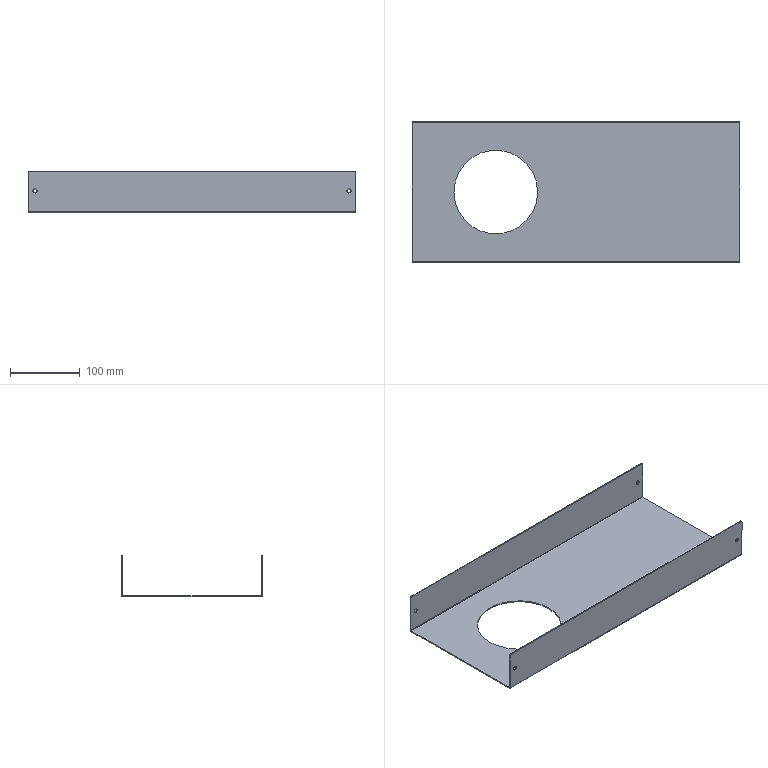Part | SolidWorks | features HoleWzd 2, Cut 1, EdgeFlange 1, Fillet 1, FlatPattern 1, SMBaseFlange 1, SheetMetal 1 | 1 solid | 36 faces | box 470 x 203 x 60 mm | volume 207704 mm3 | cylinder 18 | plane 18 | commonest cylinder face diameters 6 x8 4 x6 1 x2 120 x2
STEP:
#1=CARTESIAN_POINT('',(225.,101.5,33.));
#2=VERTEX_POINT('',#1);
#3=CARTESIAN_POINT('',(225.,101.5,27.));
#4=VERTEX_POINT('',#3);
#5=CARTESIAN_POINT('',(225.,101.5,30.));
#6=DIRECTION('',(0.,-1.,0.));
#7=DIRECTION('',(0.,0.,-1.));
#8=AXIS2_PLACEMENT_3D('',#5,#6,#7);
#9=CIRCLE('',#8,3.);
#10=EDGE_CURVE('',#2,#4,#9,.T.);
#11=ORIENTED_EDGE('',*,*,#10,.F.);
#12=CARTESIAN_POINT('',(225.,100.,33.));
#13=VERTEX_POINT('',#12);
#14=CARTESIAN_POINT('',(225.,100.,33.));
#15=DIRECTION('',(0.,-1.,0.));
#16=VECTOR('',#15,1000.);
#17=LINE('',#14,#16);
#18=EDGE_CURVE('',#2,#13,#17,.T.);
#19=ORIENTED_EDGE('',*,*,#18,.T.);
#20=CARTESIAN_POINT('',(225.,100.,27.));
#21=VERTEX_POINT('',#20);
#22=CARTESIAN_POINT('',(225.,100.,30.));
#23=DIRECTION('',(0.,-1.,0.));
#24=DIRECTION('',(0.,0.,-1.));
#25=AXIS2_PLACEMENT_3D('',#22,#23,#24);
#26=CIRCLE('',#25,3.);
#27=EDGE_CURVE('',#13,#21,#26,.T.);
#28=ORIENTED_EDGE('',*,*,#27,.T.);
#29=CARTESIAN_POINT('',(225.,100.,27.));
#30=DIRECTION('',(0.,-1.,0.));
#31=VECTOR('',#30,1000.);
#32=LINE('',#29,#31);
#33=EDGE_CURVE('',#4,#21,#32,.T.);
#34=ORIENTED_EDGE('',*,*,#33,.F.);
#35=EDGE_LOOP('',(#11,#19,#28,#34));
#36=FACE_OUTER_BOUND('',#35,.T.);
#37=CARTESIAN_POINT('',(225.,100.,30.));
#38=DIRECTION('',(0.,-1.,0.));
#39=DIRECTION('',(0.,0.,-1.));
#40=AXIS2_PLACEMENT_3D('',#37,#38,#39);
#41=CYLINDRICAL_SURFACE('',#40,3.);
#42=ADVANCED_FACE('',(#36),#41,.F.);
#43=CARTESIAN_POINT('',(-225.,101.5,33.));
#44=VERTEX_POINT('',#43);
#45=CARTESIAN_POINT('',(-225.,101.5,27.));
#46=VERTEX_POINT('',#45);
#47=CARTESIAN_POINT('',(-225.,101.5,30.));
#48=DIRECTION('',(0.,-1.,0.));
#49=DIRECTION('',(0.,0.,-1.));
#50=AXIS2_PLACEMENT_3D('',#47,#48,#49);
#51=CIRCLE('',#50,3.);
#52=EDGE_CURVE('',#44,#46,#51,.T.);
#53=ORIENTED_EDGE('',*,*,#52,.F.);
#54=CARTESIAN_POINT('',(-225.,100.,33.));
#55=VERTEX_POINT('',#54);
#56=CARTESIAN_POINT('',(-225.,100.,33.));
#57=DIRECTION('',(0.,-1.,0.));
#58=VECTOR('',#57,1000.);
#59=LINE('',#56,#58);
#60=EDGE_CURVE('',#44,#55,#59,.T.);
#61=ORIENTED_EDGE('',*,*,#60,.T.);
#62=CARTESIAN_POINT('',(-225.,100.,27.));
#63=VERTEX_POINT('',#62);
#64=CARTESIAN_POINT('',(-225.,100.,30.));
#65=DIRECTION('',(0.,-1.,0.));
#66=DIRECTION('',(0.,0.,-1.));
#67=AXIS2_PLACEMENT_3D('',#64,#65,#66);
#68=CIRCLE('',#67,3.);
#69=EDGE_CURVE('',#55,#63,#68,.T.);
#70=ORIENTED_EDGE('',*,*,#69,.T.);
#71=CARTESIAN_POINT('',(-225.,100.,27.));
#72=DIRECTION('',(0.,-1.,0.));
#73=VECTOR('',#72,1000.);
#74=LINE('',#71,#73);
#75=EDGE_CURVE('',#46,#63,#74,.T.);
#76=ORIENTED_EDGE('',*,*,#75,.F.);
#77=EDGE_LOOP('',(#53,#61,#70,#76));
#78=FACE_OUTER_BOUND('',#77,.T.);
#79=CARTESIAN_POINT('',(-225.,100.,30.));
#80=DIRECTION('',(0.,-1.,0.));
#81=DIRECTION('',(0.,0.,-1.));
#82=AXIS2_PLACEMENT_3D('',#79,#80,#81);
#83=CYLINDRICAL_SURFACE('',#82,3.);
#84=ADVANCED_FACE('',(#78),#83,.F.);
#85=CARTESIAN_POINT('',(-225.,-101.5,27.));
#86=VERTEX_POINT('',#85);
#87=CARTESIAN_POINT('',(-225.,-101.5,33.));
#88=VERTEX_POINT('',#87);
#89=CARTESIAN_POINT('',(-225.,-101.5,30.));
#90=DIRECTION('',(0.,1.,0.));
#91=DIRECTION('',(0.,0.,1.));
#92=AXIS2_PLACEMENT_3D('',#89,#90,#91);
#93=CIRCLE('',#92,3.);
#94=EDGE_CURVE('',#86,#88,#93,.T.);
#95=ORIENTED_EDGE('',*,*,#94,.F.);
#96=CARTESIAN_POINT('',(-225.,-100.,27.));
#97=VERTEX_POINT('',#96);
#98=CARTESIAN_POINT('',(-225.,-100.,27.));
#99=DIRECTION('',(0.,1.,0.));
#100=VECTOR('',#99,1000.);
#101=LINE('',#98,#100);
#102=EDGE_CURVE('',#86,#97,#101,.T.);
#103=ORIENTED_EDGE('',*,*,#102,.T.);
#104=CARTESIAN_POINT('',(-225.,-100.,33.));
#105=VERTEX_POINT('',#104);
#106=CARTESIAN_POINT('',(-225.,-100.,30.));
#107=DIRECTION('',(0.,1.,0.));
#108=DIRECTION('',(0.,0.,1.));
#109=AXIS2_PLACEMENT_3D('',#106,#107,#108);
#110=CIRCLE('',#109,3.);
#111=EDGE_CURVE('',#97,#105,#110,.T.);
#112=ORIENTED_EDGE('',*,*,#111,.T.);
#113=CARTESIAN_POINT('',(-225.,-100.,33.));
#114=DIRECTION('',(0.,1.,0.));
#115=VECTOR('',#114,1000.);
#116=LINE('',#113,#115);
#117=EDGE_CURVE('',#88,#105,#116,.T.);
#118=ORIENTED_EDGE('',*,*,#117,.F.);
#119=EDGE_LOOP('',(#95,#103,#112,#118));
#120=FACE_OUTER_BOUND('',#119,.T.);
#121=CARTESIAN_POINT('',(-225.,-100.,30.));
#122=DIRECTION('',(0.,1.,0.));
#123=DIRECTION('',(0.,0.,1.));
#124=AXIS2_PLACEMENT_3D('',#121,#122,#123);
#125=CYLINDRICAL_SURFACE('',#124,3.);
#126=ADVANCED_FACE('',(#120),#125,.F.);
#127=CARTESIAN_POINT('',(225.,-101.5,27.));
#128=VERTEX_POINT('',#127);
#129=CARTESIAN_POINT('',(225.,-101.5,33.));
#130=VERTEX_POINT('',#129);
#131=CARTESIAN_POINT('',(225.,-101.5,30.));
#132=DIRECTION('',(0.,1.,0.));
#133=DIRECTION('',(0.,0.,1.));
#134=AXIS2_PLACEMENT_3D('',#131,#132,#133);
#135=CIRCLE('',#134,3.);
#136=EDGE_CURVE('',#128,#130,#135,.T.);
#137=ORIENTED_EDGE('',*,*,#136,.F.);
#138=CARTESIAN_POINT('',(225.,-100.,27.));
#139=VERTEX_POINT('',#138);
#140=CARTESIAN_POINT('',(225.,-100.,27.));
#141=DIRECTION('',(0.,1.,0.));
#142=VECTOR('',#141,1000.);
#143=LINE('',#140,#142);
#144=EDGE_CURVE('',#128,#139,#143,.T.);
#145=ORIENTED_EDGE('',*,*,#144,.T.);
#146=CARTESIAN_POINT('',(225.,-100.,33.));
#147=VERTEX_POINT('',#146);
#148=CARTESIAN_POINT('',(225.,-100.,30.));
#149=DIRECTION('',(0.,1.,0.));
#150=DIRECTION('',(0.,0.,1.));
#151=AXIS2_PLACEMENT_3D('',#148,#149,#150);
#152=CIRCLE('',#151,3.);
#153=EDGE_CURVE('',#139,#147,#152,.T.);
#154=ORIENTED_EDGE('',*,*,#153,.T.);
#155=CARTESIAN_POINT('',(225.,-100.,33.));
#156=DIRECTION('',(0.,1.,0.));
#157=VECTOR('',#156,1000.);
#158=LINE('',#155,#157);
#159=EDGE_CURVE('',#130,#147,#158,.T.);
#160=ORIENTED_EDGE('',*,*,#159,.F.);
#161=EDGE_LOOP('',(#137,#145,#154,#160));
#162=FACE_OUTER_BOUND('',#161,.T.);
#163=CARTESIAN_POINT('',(225.,-100.,30.));
#164=DIRECTION('',(0.,1.,0.));
#165=DIRECTION('',(0.,0.,1.));
#166=AXIS2_PLACEMENT_3D('',#163,#164,#165);
#167=CYLINDRICAL_SURFACE('',#166,3.);
#168=ADVANCED_FACE('',(#162),#167,.F.);
#169=CARTESIAN_POINT('',(-175.,0.,0.));
#170=VERTEX_POINT('',#169);
#171=CARTESIAN_POINT('',(-55.,0.,0.));
#172=VERTEX_POINT('',#171);
#173=CARTESIAN_POINT('',(-115.,0.,0.));
#174=DIRECTION('',(0.,0.,1.));
#175=DIRECTION('',(1.,0.,0.));
#176=AXIS2_PLACEMENT_3D('',#173,#174,#175);
#177=CIRCLE('',#176,60.);
#178=EDGE_CURVE('',#170,#172,#177,.T.);
#179=ORIENTED_EDGE('',*,*,#178,.T.);
#180=CARTESIAN_POINT('',(-55.,0.,-1.5));
#181=VERTEX_POINT('',#180);
#182=CARTESIAN_POINT('',(-55.,0.,8.5));
#183=DIRECTION('',(0.,0.,-1.));
#184=VECTOR('',#183,1000.);
#185=LINE('',#182,#184);
#186=EDGE_CURVE('',#172,#181,#185,.T.);
#187=ORIENTED_EDGE('',*,*,#186,.T.);
#188=CARTESIAN_POINT('',(-175.,0.,-1.5));
#189=VERTEX_POINT('',#188);
#190=CARTESIAN_POINT('',(-115.,0.,-1.5));
#191=DIRECTION('',(0.,0.,-1.));
#192=DIRECTION('',(-1.,0.,0.));
#193=AXIS2_PLACEMENT_3D('',#190,#191,#192);
#194=CIRCLE('',#193,60.);
#195=EDGE_CURVE('',#181,#189,#194,.T.);
#196=ORIENTED_EDGE('',*,*,#195,.T.);
#197=CARTESIAN_POINT('',(-175.,0.,8.5));
#198=DIRECTION('',(0.,0.,-1.));
#199=VECTOR('',#198,1000.);
#200=LINE('',#197,#199);
#201=EDGE_CURVE('',#170,#189,#200,.T.);
#202=ORIENTED_EDGE('',*,*,#201,.F.);
#203=EDGE_LOOP('',(#179,#187,#196,#202));
#204=FACE_OUTER_BOUND('',#203,.T.);
#205=CARTESIAN_POINT('',(-115.,0.,8.5));
#206=DIRECTION('',(0.,0.,-1.));
#207=DIRECTION('',(-1.,0.,0.));
#208=AXIS2_PLACEMENT_3D('',#205,#206,#207);
#209=CYLINDRICAL_SURFACE('',#208,60.);
#210=ADVANCED_FACE('',(#204),#209,.F.);
#211=CARTESIAN_POINT('',(-115.,0.,-1.5));
#212=DIRECTION('',(0.,0.,-1.));
#213=DIRECTION('',(-1.,0.,0.));
#214=AXIS2_PLACEMENT_3D('',#211,#212,#213);
#215=CIRCLE('',#214,60.);
#216=EDGE_CURVE('',#189,#181,#215,.T.);
#217=ORIENTED_EDGE('',*,*,#216,.F.);
#218=ORIENTED_EDGE('',*,*,#195,.F.);
#219=EDGE_LOOP('',(#217,#218));
#220=FACE_BOUND('',#219,.T.);
#221=CARTESIAN_POINT('',(235.,-99.5,-1.5));
#222=VERTEX_POINT('',#221);
#223=CARTESIAN_POINT('',(-235.,-99.5,-1.5));
#224=VERTEX_POINT('',#223);
#225=CARTESIAN_POINT('',(235.,-99.5,-1.5));
#226=DIRECTION('',(-1.,0.,0.));
#227=VECTOR('',#226,1000.);
#228=LINE('',#225,#227);
#229=EDGE_CURVE('',#222,#224,#228,.T.);
#230=ORIENTED_EDGE('',*,*,#229,.T.);
#231=CARTESIAN_POINT('',(-235.,99.5,-1.5));
#232=VERTEX_POINT('',#231);
#233=CARTESIAN_POINT('',(-235.,100.,-1.5));
#234=DIRECTION('',(0.,-1.,0.));
#235=VECTOR('',#234,1000.);
#236=LINE('',#233,#235);
#237=EDGE_CURVE('',#232,#224,#236,.T.);
#238=ORIENTED_EDGE('',*,*,#237,.F.);
#239=CARTESIAN_POINT('',(235.,99.5,-1.5));
#240=VERTEX_POINT('',#239);
#241=CARTESIAN_POINT('',(-235.,99.5,-1.5));
#242=DIRECTION('',(1.,0.,0.));
#243=VECTOR('',#242,1000.);
#244=LINE('',#241,#243);
#245=EDGE_CURVE('',#232,#240,#244,.T.);
#246=ORIENTED_EDGE('',*,*,#245,.T.);
#247=CARTESIAN_POINT('',(235.,100.,-1.5));
#248=DIRECTION('',(0.,1.,0.));
#249=VECTOR('',#248,1000.);
#250=LINE('',#247,#249);
#251=EDGE_CURVE('',#222,#240,#250,.T.);
#252=ORIENTED_EDGE('',*,*,#251,.F.);
#253=EDGE_LOOP('',(#230,#238,#246,#252));
#254=FACE_OUTER_BOUND('',#253,.T.);
#255=CARTESIAN_POINT('',(0.,0.,-1.5));
#256=DIRECTION('',(0.,0.,1.));
#257=DIRECTION('',(1.,0.,0.));
#258=AXIS2_PLACEMENT_3D('',#255,#256,#257);
#259=PLANE('',#258);
#260=ADVANCED_FACE('',(#220,#254),#259,.F.);
#261=ORIENTED_EDGE('',*,*,#178,.F.);
#262=CARTESIAN_POINT('',(-115.,0.,0.));
#263=DIRECTION('',(0.,0.,1.));
#264=DIRECTION('',(1.,0.,0.));
#265=AXIS2_PLACEMENT_3D('',#262,#263,#264);
#266=CIRCLE('',#265,60.);
#267=EDGE_CURVE('',#172,#170,#266,.T.);
#268=ORIENTED_EDGE('',*,*,#267,.F.);
#269=EDGE_LOOP('',(#261,#268));
#270=FACE_BOUND('',#269,.T.);
#271=CARTESIAN_POINT('',(-235.,99.5,0.));
#272=VERTEX_POINT('',#271);
#273=CARTESIAN_POINT('',(-235.,-99.5,0.));
#274=VERTEX_POINT('',#273);
#275=CARTESIAN_POINT('',(-235.,100.,0.));
#276=DIRECTION('',(0.,-1.,0.));
#277=VECTOR('',#276,1000.);
#278=LINE('',#275,#277);
#279=EDGE_CURVE('',#272,#274,#278,.T.);
#280=ORIENTED_EDGE('',*,*,#279,.T.);
#281=CARTESIAN_POINT('',(235.,-99.5,0.));
#282=VERTEX_POINT('',#281);
#283=CARTESIAN_POINT('',(235.,-99.5,0.));
#284=DIRECTION('',(-1.,0.,0.));
#285=VECTOR('',#284,1000.);
#286=LINE('',#283,#285);
#287=EDGE_CURVE('',#282,#274,#286,.T.);
#288=ORIENTED_EDGE('',*,*,#287,.F.);
#289=CARTESIAN_POINT('',(235.,99.5,0.));
#290=VERTEX_POINT('',#289);
#291=CARTESIAN_POINT('',(235.,100.,0.));
#292=DIRECTION('',(0.,1.,0.));
#293=VECTOR('',#292,1000.);
#294=LINE('',#291,#293);
#295=EDGE_CURVE('',#282,#290,#294,.T.);
#296=ORIENTED_EDGE('',*,*,#295,.T.);
#297=CARTESIAN_POINT('',(-235.,99.5,0.));
#298=DIRECTION('',(1.,0.,0.));
#299=VECTOR('',#298,1000.);
#300=LINE('',#297,#299);
#301=EDGE_CURVE('',#272,#290,#300,.T.);
#302=ORIENTED_EDGE('',*,*,#301,.F.);
#303=EDGE_LOOP('',(#280,#288,#296,#302));
#304=FACE_OUTER_BOUND('',#303,.T.);
#305=CARTESIAN_POINT('',(0.,0.,0.));
#306=DIRECTION('',(0.,0.,1.));
#307=DIRECTION('',(1.,0.,0.));
#308=AXIS2_PLACEMENT_3D('',#305,#306,#307);
#309=PLANE('',#308);
#310=ADVANCED_FACE('',(#270,#304),#309,.T.);
#311=ORIENTED_EDGE('',*,*,#295,.F.);
#312=CARTESIAN_POINT('',(235.,-99.5,0.));
#313=DIRECTION('',(0.,0.,-1.));
#314=VECTOR('',#313,1000.);
#315=LINE('',#312,#314);
#316=EDGE_CURVE('',#282,#222,#315,.T.);
#317=ORIENTED_EDGE('',*,*,#316,.T.);
#318=ORIENTED_EDGE('',*,*,#251,.T.);
#319=CARTESIAN_POINT('',(235.,99.5,0.));
#320=DIRECTION('',(0.,0.,-1.));
#321=VECTOR('',#320,1000.);
#322=LINE('',#319,#321);
#323=EDGE_CURVE('',#290,#240,#322,.T.);
#324=ORIENTED_EDGE('',*,*,#323,.F.);
#325=EDGE_LOOP('',(#311,#317,#318,#324));
#326=FACE_OUTER_BOUND('',#325,.T.);
#327=CARTESIAN_POINT('',(235.,100.,-1.5));
#328=DIRECTION('',(1.,0.,0.));
#329=DIRECTION('',(0.,1.,0.));
#330=AXIS2_PLACEMENT_3D('',#327,#328,#329);
#331=PLANE('',#330);
#332=ADVANCED_FACE('',(#326),#331,.T.);
#333=CARTESIAN_POINT('',(-235.,-99.5,0.));
#334=DIRECTION('',(0.,0.,-1.));
#335=VECTOR('',#334,1000.);
#336=LINE('',#333,#335);
#337=EDGE_CURVE('',#274,#224,#336,.T.);
#338=ORIENTED_EDGE('',*,*,#337,.F.);
#339=ORIENTED_EDGE('',*,*,#279,.F.);
#340=CARTESIAN_POINT('',(-235.,99.5,0.));
#341=DIRECTION('',(0.,0.,-1.));
#342=VECTOR('',#341,1000.);
#343=LINE('',#340,#342);
#344=EDGE_CURVE('',#272,#232,#343,.T.);
#345=ORIENTED_EDGE('',*,*,#344,.T.);
#346=ORIENTED_EDGE('',*,*,#237,.T.);
#347=EDGE_LOOP('',(#338,#339,#345,#346));
#348=FACE_OUTER_BOUND('',#347,.T.);
#349=CARTESIAN_POINT('',(-235.,100.,-1.5));
#350=DIRECTION('',(-1.,0.,0.));
#351=DIRECTION('',(0.,-1.,0.));
#352=AXIS2_PLACEMENT_3D('',#349,#350,#351);
#353=PLANE('',#352);
#354=ADVANCED_FACE('',(#348),#353,.T.);
#355=CARTESIAN_POINT('',(235.,100.,0.5));
#356=VERTEX_POINT('',#355);
#357=CARTESIAN_POINT('',(235.,101.5,0.5));
#358=VERTEX_POINT('',#357);
#359=CARTESIAN_POINT('',(235.,100.,0.5));
#360=DIRECTION('',(0.,1.,0.));
#361=VECTOR('',#360,1000.);
#362=LINE('',#359,#361);
#363=EDGE_CURVE('',#356,#358,#362,.T.);
#364=ORIENTED_EDGE('',*,*,#363,.F.);
#365=CARTESIAN_POINT('',(235.,99.5,0.5));
#366=DIRECTION('',(1.,0.,0.));
#367=DIRECTION('',(0.,0.,1.));
#368=AXIS2_PLACEMENT_3D('',#365,#366,#367);
#369=CIRCLE('',#368,0.5);
#370=EDGE_CURVE('',#290,#356,#369,.T.);
#371=ORIENTED_EDGE('',*,*,#370,.F.);
#372=ORIENTED_EDGE('',*,*,#323,.T.);
#373=CARTESIAN_POINT('',(235.,99.5,0.5));
#374=DIRECTION('',(1.,0.,0.));
#375=DIRECTION('',(0.,0.,1.));
#376=AXIS2_PLACEMENT_3D('',#373,#374,#375);
#377=CIRCLE('',#376,2.);
#378=EDGE_CURVE('',#240,#358,#377,.T.);
#379=ORIENTED_EDGE('',*,*,#378,.T.);
#380=EDGE_LOOP('',(#364,#371,#372,#379));
#381=FACE_OUTER_BOUND('',#380,.T.);
#382=CARTESIAN_POINT('',(235.,99.5,0.5));
#383=DIRECTION('',(1.,0.,0.));
#384=DIRECTION('',(0.,0.,-1.));
#385=AXIS2_PLACEMENT_3D('',#382,#383,#384);
#386=PLANE('',#385);
#387=ADVANCED_FACE('',(#381),#386,.T.);
#388=CARTESIAN_POINT('',(-235.,100.,0.5));
#389=VERTEX_POINT('',#388);
#390=CARTESIAN_POINT('',(-235.,99.5,0.5));
#391=DIRECTION('',(-1.,0.,0.));
#392=DIRECTION('',(0.,0.,1.));
#393=AXIS2_PLACEMENT_3D('',#390,#391,#392);
#394=CIRCLE('',#393,0.5);
#395=EDGE_CURVE('',#389,#272,#394,.T.);
#396=ORIENTED_EDGE('',*,*,#395,.F.);
#397=CARTESIAN_POINT('',(-235.,101.5,0.5));
#398=VERTEX_POINT('',#397);
#399=CARTESIAN_POINT('',(-235.,100.,0.5));
#400=DIRECTION('',(0.,1.,0.));
#401=VECTOR('',#400,1000.);
#402=LINE('',#399,#401);
#403=EDGE_CURVE('',#389,#398,#402,.T.);
#404=ORIENTED_EDGE('',*,*,#403,.T.);
#405=CARTESIAN_POINT('',(-235.,99.5,0.5));
#406=DIRECTION('',(-1.,0.,0.));
#407=DIRECTION('',(0.,0.,1.));
#408=AXIS2_PLACEMENT_3D('',#405,#406,#407);
#409=CIRCLE('',#408,2.);
#410=EDGE_CURVE('',#398,#232,#409,.T.);
#411=ORIENTED_EDGE('',*,*,#410,.T.);
#412=ORIENTED_EDGE('',*,*,#344,.F.);
#413=EDGE_LOOP('',(#396,#404,#411,#412));
#414=FACE_OUTER_BOUND('',#413,.T.);
#415=CARTESIAN_POINT('',(-235.,99.5,0.5));
#416=DIRECTION('',(1.,0.,0.));
#417=DIRECTION('',(0.,0.,-1.));
#418=AXIS2_PLACEMENT_3D('',#415,#416,#417);
#419=PLANE('',#418);
#420=ADVANCED_FACE('',(#414),#419,.F.);
#421=ORIENTED_EDGE('',*,*,#245,.F.);
#422=ORIENTED_EDGE('',*,*,#410,.F.);
#423=CARTESIAN_POINT('',(0.,101.5,0.5));
#424=DIRECTION('',(-1.,0.,0.));
#425=VECTOR('',#424,1000.);
#426=LINE('',#423,#425);
#427=EDGE_CURVE('',#358,#398,#426,.T.);
#428=ORIENTED_EDGE('',*,*,#427,.F.);
#429=ORIENTED_EDGE('',*,*,#378,.F.);
#430=EDGE_LOOP('',(#421,#422,#428,#429));
#431=FACE_OUTER_BOUND('',#430,.T.);
#432=CARTESIAN_POINT('',(-235.,99.5,0.5));
#433=DIRECTION('',(-1.,0.,0.));
#434=DIRECTION('',(0.,1.,0.));
#435=AXIS2_PLACEMENT_3D('',#432,#433,#434);
#436=CYLINDRICAL_SURFACE('',#435,2.);
#437=ADVANCED_FACE('',(#431),#436,.T.);
#438=ORIENTED_EDGE('',*,*,#301,.T.);
#439=ORIENTED_EDGE('',*,*,#370,.T.);
#440=CARTESIAN_POINT('',(235.,100.,0.5));
#441=DIRECTION('',(-1.,0.,0.));
#442=VECTOR('',#441,1000.);
#443=LINE('',#440,#442);
#444=EDGE_CURVE('',#356,#389,#443,.T.);
#445=ORIENTED_EDGE('',*,*,#444,.T.);
#446=ORIENTED_EDGE('',*,*,#395,.T.);
#447=EDGE_LOOP('',(#438,#439,#445,#446));
#448=FACE_OUTER_BOUND('',#447,.T.);
#449=CARTESIAN_POINT('',(-235.,99.5,0.5));
#450=DIRECTION('',(-1.,0.,0.));
#451=DIRECTION('',(0.,1.,0.));
#452=AXIS2_PLACEMENT_3D('',#449,#450,#451);
#453=CYLINDRICAL_SURFACE('',#452,0.5);
#454=ADVANCED_FACE('',(#448),#453,.F.);
#455=CARTESIAN_POINT('',(-235.,100.,56.5));
#456=VERTEX_POINT('',#455);
#457=CARTESIAN_POINT('',(-235.,100.,0.));
#458=DIRECTION('',(0.,0.,-1.));
#459=VECTOR('',#458,1000.);
#460=LINE('',#457,#459);
#461=EDGE_CURVE('',#456,#389,#460,.T.);
#462=ORIENTED_EDGE('',*,*,#461,.F.);
#463=CARTESIAN_POINT('',(-235.,101.5,56.5));
#464=VERTEX_POINT('',#463);
#465=CARTESIAN_POINT('',(-235.,101.5,56.5));
#466=DIRECTION('',(0.,1.,0.));
#467=VECTOR('',#466,1000.);
#468=LINE('',#465,#467);
#469=EDGE_CURVE('',#456,#464,#468,.T.);
#470=ORIENTED_EDGE('',*,*,#469,.T.);
#471=CARTESIAN_POINT('',(-235.,101.5,0.));
#472=DIRECTION('',(0.,0.,-1.));
#473=VECTOR('',#472,1000.);
#474=LINE('',#471,#473);
#475=EDGE_CURVE('',#464,#398,#474,.T.);
#476=ORIENTED_EDGE('',*,*,#475,.T.);
#477=ORIENTED_EDGE('',*,*,#403,.F.);
#478=EDGE_LOOP('',(#462,#470,#476,#477));
#479=FACE_OUTER_BOUND('',#478,.T.);
#480=CARTESIAN_POINT('',(-235.,101.5,0.));
#481=DIRECTION('',(-1.,0.,0.));
#482=DIRECTION('',(0.,0.,1.));
#483=AXIS2_PLACEMENT_3D('',#480,#481,#482);
#484=PLANE('',#483);
#485=ADVANCED_FACE('',(#479),#484,.T.);
#486=CARTESIAN_POINT('',(235.,101.5,56.5));
#487=VERTEX_POINT('',#486);
#488=CARTESIAN_POINT('',(235.,101.5,58.5));
#489=DIRECTION('',(0.,0.,1.));
#490=VECTOR('',#489,1000.);
#491=LINE('',#488,#490);
#492=EDGE_CURVE('',#358,#487,#491,.T.);
#493=ORIENTED_EDGE('',*,*,#492,.T.);
#494=CARTESIAN_POINT('',(235.,100.,56.5));
#495=VERTEX_POINT('',#494);
#496=CARTESIAN_POINT('',(235.,101.5,56.5));
#497=DIRECTION('',(0.,-1.,0.));
#498=VECTOR('',#497,1000.);
#499=LINE('',#496,#498);
#500=EDGE_CURVE('',#487,#495,#499,.T.);
#501=ORIENTED_EDGE('',*,*,#500,.T.);
#502=CARTESIAN_POINT('',(235.,100.,58.5));
#503=DIRECTION('',(0.,0.,1.));
#504=VECTOR('',#503,1000.);
#505=LINE('',#502,#504);
#506=EDGE_CURVE('',#356,#495,#505,.T.);
#507=ORIENTED_EDGE('',*,*,#506,.F.);
#508=ORIENTED_EDGE('',*,*,#363,.T.);
#509=EDGE_LOOP('',(#493,#501,#507,#508));
#510=FACE_OUTER_BOUND('',#509,.T.);
#511=CARTESIAN_POINT('',(235.,101.5,58.5));
#512=DIRECTION('',(1.,0.,0.));
#513=DIRECTION('',(0.,0.,-1.));
#514=AXIS2_PLACEMENT_3D('',#511,#512,#513);
#515=PLANE('',#514);
#516=ADVANCED_FACE('',(#510),#515,.T.);
#517=CARTESIAN_POINT('',(225.,101.5,30.));
#518=DIRECTION('',(0.,-1.,0.));
#519=DIRECTION('',(0.,0.,-1.));
#520=AXIS2_PLACEMENT_3D('',#517,#518,#519);
#521=CIRCLE('',#520,3.);
#522=EDGE_CURVE('',#4,#2,#521,.T.);
#523=ORIENTED_EDGE('',*,*,#522,.T.);
#524=ORIENTED_EDGE('',*,*,#10,.T.);
#525=EDGE_LOOP('',(#523,#524));
#526=FACE_BOUND('',#525,.T.);
#527=CARTESIAN_POINT('',(-225.,101.5,30.));
#528=DIRECTION('',(0.,-1.,0.));
#529=DIRECTION('',(0.,0.,-1.));
#530=AXIS2_PLACEMENT_3D('',#527,#528,#529);
#531=CIRCLE('',#530,3.);
#532=EDGE_CURVE('',#46,#44,#531,.T.);
#533=ORIENTED_EDGE('',*,*,#532,.T.);
#534=ORIENTED_EDGE('',*,*,#52,.T.);
#535=EDGE_LOOP('',(#533,#534));
#536=FACE_BOUND('',#535,.T.);
#537=CARTESIAN_POINT('',(233.,101.5,58.5));
#538=VERTEX_POINT('',#537);
#539=CARTESIAN_POINT('',(-233.,101.5,58.5));
#540=VERTEX_POINT('',#539);
#541=CARTESIAN_POINT('',(-235.,101.5,58.5));
#542=DIRECTION('',(-1.,0.,0.));
#543=VECTOR('',#542,1000.);
#544=LINE('',#541,#543);
#545=EDGE_CURVE('',#538,#540,#544,.T.);
#546=ORIENTED_EDGE('',*,*,#545,.F.);
#547=CARTESIAN_POINT('',(233.,101.5,56.5));
#548=DIRECTION('',(0.,1.,0.));
#549=DIRECTION('',(0.,0.,1.));
#550=AXIS2_PLACEMENT_3D('',#547,#548,#549);
#551=CIRCLE('',#550,2.);
#552=EDGE_CURVE('',#538,#487,#551,.T.);
#553=ORIENTED_EDGE('',*,*,#552,.T.);
#554=ORIENTED_EDGE('',*,*,#492,.F.);
#555=ORIENTED_EDGE('',*,*,#427,.T.);
#556=ORIENTED_EDGE('',*,*,#475,.F.);
#557=CARTESIAN_POINT('',(-233.,101.5,56.5));
#558=DIRECTION('',(0.,1.,0.));
#559=DIRECTION('',(0.,0.,1.));
#560=AXIS2_PLACEMENT_3D('',#557,#558,#559);
#561=CIRCLE('',#560,2.);
#562=EDGE_CURVE('',#464,#540,#561,.T.);
#563=ORIENTED_EDGE('',*,*,#562,.T.);
#564=EDGE_LOOP('',(#546,#553,#554,#555,#556,#563));
#565=FACE_OUTER_BOUND('',#564,.T.);
#566=CARTESIAN_POINT('',(0.,101.5,0.));
#567=DIRECTION('',(0.,1.,0.));
#568=DIRECTION('',(0.,0.,1.));
#569=AXIS2_PLACEMENT_3D('',#566,#567,#568);
#570=PLANE('',#569);
#571=ADVANCED_FACE('',(#526,#536,#565),#570,.T.);
#572=CARTESIAN_POINT('',(225.,100.,30.));
#573=DIRECTION('',(0.,-1.,0.));
#574=DIRECTION('',(0.,0.,-1.));
#575=AXIS2_PLACEMENT_3D('',#572,#573,#574);
#576=CIRCLE('',#575,3.);
#577=EDGE_CURVE('',#21,#13,#576,.T.);
#578=ORIENTED_EDGE('',*,*,#577,.F.);
#579=ORIENTED_EDGE('',*,*,#27,.F.);
#580=EDGE_LOOP('',(#578,#579));
#581=FACE_BOUND('',#580,.T.);
#582=CARTESIAN_POINT('',(-225.,100.,30.));
#583=DIRECTION('',(0.,-1.,0.));
#584=DIRECTION('',(0.,0.,-1.));
#585=AXIS2_PLACEMENT_3D('',#582,#583,#584);
#586=CIRCLE('',#585,3.);
#587=EDGE_CURVE('',#63,#55,#586,.T.);
#588=ORIENTED_EDGE('',*,*,#587,.F.);
#589=ORIENTED_EDGE('',*,*,#69,.F.);
#590=EDGE_LOOP('',(#588,#589));
#591=FACE_BOUND('',#590,.T.);
#592=ORIENTED_EDGE('',*,*,#506,.T.);
#593=CARTESIAN_POINT('',(233.,100.,58.5));
#594=VERTEX_POINT('',#593);
#595=CARTESIAN_POINT('',(233.,100.,56.5));
#596=DIRECTION('',(0.,-1.,0.));
#597=DIRECTION('',(0.,0.,1.));
#598=AXIS2_PLACEMENT_3D('',#595,#596,#597);
#599=CIRCLE('',#598,2.);
#600=EDGE_CURVE('',#495,#594,#599,.T.);
#601=ORIENTED_EDGE('',*,*,#600,.T.);
#602=CARTESIAN_POINT('',(-233.,100.,58.5));
#603=VERTEX_POINT('',#602);
#604=CARTESIAN_POINT('',(-235.,100.,58.5));
#605=DIRECTION('',(-1.,0.,0.));
#606=VECTOR('',#605,1000.);
#607=LINE('',#604,#606);
#608=EDGE_CURVE('',#594,#603,#607,.T.);
#609=ORIENTED_EDGE('',*,*,#608,.T.);
#610=CARTESIAN_POINT('',(-233.,100.,56.5));
#611=DIRECTION('',(0.,-1.,0.));
#612=DIRECTION('',(0.,0.,1.));
#613=AXIS2_PLACEMENT_3D('',#610,#611,#612);
#614=CIRCLE('',#613,2.);
#615=EDGE_CURVE('',#603,#456,#614,.T.);
#616=ORIENTED_EDGE('',*,*,#615,.T.);
#617=ORIENTED_EDGE('',*,*,#461,.T.);
#618=ORIENTED_EDGE('',*,*,#444,.F.);
#619=EDGE_LOOP('',(#592,#601,#609,#616,#617,#618));
#620=FACE_OUTER_BOUND('',#619,.T.);
#621=CARTESIAN_POINT('',(0.,100.,0.));
#622=DIRECTION('',(0.,1.,0.));
#623=DIRECTION('',(0.,0.,1.));
#624=AXIS2_PLACEMENT_3D('',#621,#622,#623);
#625=PLANE('',#624);
#626=ADVANCED_FACE('',(#581,#591,#620),#625,.F.);
#627=ORIENTED_EDGE('',*,*,#608,.F.);
#628=CARTESIAN_POINT('',(233.,101.5,58.5));
#629=DIRECTION('',(0.,1.,0.));
#630=VECTOR('',#629,1000.);
#631=LINE('',#628,#630);
#632=EDGE_CURVE('',#594,#538,#631,.T.);
#633=ORIENTED_EDGE('',*,*,#632,.T.);
#634=ORIENTED_EDGE('',*,*,#545,.T.);
#635=CARTESIAN_POINT('',(-233.,101.5,58.5));
#636=DIRECTION('',(0.,-1.,0.));
#637=VECTOR('',#636,1000.);
#638=LINE('',#635,#637);
#639=EDGE_CURVE('',#540,#603,#638,.T.);
#640=ORIENTED_EDGE('',*,*,#639,.T.);
#641=EDGE_LOOP('',(#627,#633,#634,#640));
#642=FACE_OUTER_BOUND('',#641,.T.);
#643=CARTESIAN_POINT('',(-235.,101.5,58.5));
#644=DIRECTION('',(0.,0.,1.));
#645=DIRECTION('',(0.,-1.,0.));
#646=AXIS2_PLACEMENT_3D('',#643,#644,#645);
#647=PLANE('',#646);
#648=ADVANCED_FACE('',(#642),#647,.T.);
#649=CARTESIAN_POINT('',(-235.,-100.,0.5));
#650=VERTEX_POINT('',#649);
#651=CARTESIAN_POINT('',(-235.,-101.5,0.5));
#652=VERTEX_POINT('',#651);
#653=CARTESIAN_POINT('',(-235.,-100.,0.5));
#654=DIRECTION('',(0.,-1.,0.));
#655=VECTOR('',#654,1000.);
#656=LINE('',#653,#655);
#657=EDGE_CURVE('',#650,#652,#656,.T.);
#658=ORIENTED_EDGE('',*,*,#657,.F.);
#659=CARTESIAN_POINT('',(-235.,-99.5,0.5));
#660=DIRECTION('',(-1.,0.,0.));
#661=DIRECTION('',(0.,0.,-1.));
#662=AXIS2_PLACEMENT_3D('',#659,#660,#661);
#663=CIRCLE('',#662,0.5);
#664=EDGE_CURVE('',#274,#650,#663,.T.);
#665=ORIENTED_EDGE('',*,*,#664,.F.);
#666=ORIENTED_EDGE('',*,*,#337,.T.);
#667=CARTESIAN_POINT('',(-235.,-99.5,0.5));
#668=DIRECTION('',(-1.,0.,0.));
#669=DIRECTION('',(0.,0.,-1.));
#670=AXIS2_PLACEMENT_3D('',#667,#668,#669);
#671=CIRCLE('',#670,2.);
#672=EDGE_CURVE('',#224,#652,#671,.T.);
#673=ORIENTED_EDGE('',*,*,#672,.T.);
#674=EDGE_LOOP('',(#658,#665,#666,#673));
#675=FACE_OUTER_BOUND('',#674,.T.);
#676=CARTESIAN_POINT('',(-235.,-99.5,0.5));
#677=DIRECTION('',(-1.,0.,0.));
#678=DIRECTION('',(0.,0.,1.));
#679=AXIS2_PLACEMENT_3D('',#676,#677,#678);
#680=PLANE('',#679);
#681=ADVANCED_FACE('',(#675),#680,.T.);
#682=CARTESIAN_POINT('',(235.,-100.,0.5));
#683=VERTEX_POINT('',#682);
#684=CARTESIAN_POINT('',(235.,-99.5,0.5));
#685=DIRECTION('',(1.,0.,0.));
#686=DIRECTION('',(0.,0.,-1.));
#687=AXIS2_PLACEMENT_3D('',#684,#685,#686);
#688=CIRCLE('',#687,0.5);
#689=EDGE_CURVE('',#683,#282,#688,.T.);
#690=ORIENTED_EDGE('',*,*,#689,.F.);
#691=CARTESIAN_POINT('',(235.,-101.5,0.5));
#692=VERTEX_POINT('',#691);
#693=CARTESIAN_POINT('',(235.,-100.,0.5));
#694=DIRECTION('',(0.,-1.,0.));
#695=VECTOR('',#694,1000.);
#696=LINE('',#693,#695);
#697=EDGE_CURVE('',#683,#692,#696,.T.);
#698=ORIENTED_EDGE('',*,*,#697,.T.);
#699=CARTESIAN_POINT('',(235.,-99.5,0.5));
#700=DIRECTION('',(1.,0.,0.));
#701=DIRECTION('',(0.,0.,-1.));
#702=AXIS2_PLACEMENT_3D('',#699,#700,#701);
#703=CIRCLE('',#702,2.);
#704=EDGE_CURVE('',#692,#222,#703,.T.);
#705=ORIENTED_EDGE('',*,*,#704,.T.);
#706=ORIENTED_EDGE('',*,*,#316,.F.);
#707=EDGE_LOOP('',(#690,#698,#705,#706));
#708=FACE_OUTER_BOUND('',#707,.T.);
#709=CARTESIAN_POINT('',(235.,-99.5,0.5));
#710=DIRECTION('',(-1.,0.,0.));
#711=DIRECTION('',(0.,0.,1.));
#712=AXIS2_PLACEMENT_3D('',#709,#710,#711);
#713=PLANE('',#712);
#714=ADVANCED_FACE('',(#708),#713,.F.);
#715=ORIENTED_EDGE('',*,*,#229,.F.);
#716=ORIENTED_EDGE('',*,*,#704,.F.);
#717=CARTESIAN_POINT('',(0.,-101.5,0.5));
#718=DIRECTION('',(-1.,0.,0.));
#719=VECTOR('',#718,1000.);
#720=LINE('',#717,#719);
#721=EDGE_CURVE('',#692,#652,#720,.T.);
#722=ORIENTED_EDGE('',*,*,#721,.T.);
#723=ORIENTED_EDGE('',*,*,#672,.F.);
#724=EDGE_LOOP('',(#715,#716,#722,#723));
#725=FACE_OUTER_BOUND('',#724,.T.);
#726=CARTESIAN_POINT('',(235.,-99.5,0.5));
#727=DIRECTION('',(1.,0.,0.));
#728=DIRECTION('',(0.,-1.,0.));
#729=AXIS2_PLACEMENT_3D('',#726,#727,#728);
#730=CYLINDRICAL_SURFACE('',#729,2.);
#731=ADVANCED_FACE('',(#725),#730,.T.);
#732=ORIENTED_EDGE('',*,*,#287,.T.);
#733=ORIENTED_EDGE('',*,*,#664,.T.);
#734=CARTESIAN_POINT('',(-235.,-100.,0.5));
#735=DIRECTION('',(1.,0.,0.));
#736=VECTOR('',#735,1000.);
#737=LINE('',#734,#736);
#738=EDGE_CURVE('',#650,#683,#737,.T.);
#739=ORIENTED_EDGE('',*,*,#738,.T.);
#740=ORIENTED_EDGE('',*,*,#689,.T.);
#741=EDGE_LOOP('',(#732,#733,#739,#740));
#742=FACE_OUTER_BOUND('',#741,.T.);
#743=CARTESIAN_POINT('',(235.,-99.5,0.5));
#744=DIRECTION('',(1.,0.,0.));
#745=DIRECTION('',(0.,-1.,0.));
#746=AXIS2_PLACEMENT_3D('',#743,#744,#745);
#747=CYLINDRICAL_SURFACE('',#746,0.5);
#748=ADVANCED_FACE('',(#742),#747,.F.);
#749=CARTESIAN_POINT('',(-235.,-101.5,56.5));
#750=VERTEX_POINT('',#749);
#751=CARTESIAN_POINT('',(-235.,-101.5,0.));
#752=DIRECTION('',(0.,0.,1.));
#753=VECTOR('',#752,1000.);
#754=LINE('',#751,#753);
#755=EDGE_CURVE('',#652,#750,#754,.T.);
#756=ORIENTED_EDGE('',*,*,#755,.T.);
#757=CARTESIAN_POINT('',(-235.,-100.,56.5));
#758=VERTEX_POINT('',#757);
#759=CARTESIAN_POINT('',(-235.,-101.5,56.5));
#760=DIRECTION('',(0.,1.,0.));
#761=VECTOR('',#760,1000.);
#762=LINE('',#759,#761);
#763=EDGE_CURVE('',#750,#758,#762,.T.);
#764=ORIENTED_EDGE('',*,*,#763,.T.);
#765=CARTESIAN_POINT('',(-235.,-100.,0.));
#766=DIRECTION('',(0.,0.,1.));
#767=VECTOR('',#766,1000.);
#768=LINE('',#765,#767);
#769=EDGE_CURVE('',#650,#758,#768,.T.);
#770=ORIENTED_EDGE('',*,*,#769,.F.);
#771=ORIENTED_EDGE('',*,*,#657,.T.);
#772=EDGE_LOOP('',(#756,#764,#770,#771));
#773=FACE_OUTER_BOUND('',#772,.T.);
#774=CARTESIAN_POINT('',(-235.,-101.5,0.));
#775=DIRECTION('',(-1.,0.,0.));
#776=DIRECTION('',(0.,0.,1.));
#777=AXIS2_PLACEMENT_3D('',#774,#775,#776);
#778=PLANE('',#777);
#779=ADVANCED_FACE('',(#773),#778,.T.);
#780=CARTESIAN_POINT('',(235.,-100.,56.5));
#781=VERTEX_POINT('',#780);
#782=CARTESIAN_POINT('',(235.,-100.,58.5));
#783=DIRECTION('',(0.,0.,-1.));
#784=VECTOR('',#783,1000.);
#785=LINE('',#782,#784);
#786=EDGE_CURVE('',#781,#683,#785,.T.);
#787=ORIENTED_EDGE('',*,*,#786,.F.);
#788=CARTESIAN_POINT('',(235.,-101.5,56.5));
#789=VERTEX_POINT('',#788);
#790=CARTESIAN_POINT('',(235.,-101.5,56.5));
#791=DIRECTION('',(0.,-1.,0.));
#792=VECTOR('',#791,1000.);
#793=LINE('',#790,#792);
#794=EDGE_CURVE('',#781,#789,#793,.T.);
#795=ORIENTED_EDGE('',*,*,#794,.T.);
#796=CARTESIAN_POINT('',(235.,-101.5,58.5));
#797=DIRECTION('',(0.,0.,-1.));
#798=VECTOR('',#797,1000.);
#799=LINE('',#796,#798);
#800=EDGE_CURVE('',#789,#692,#799,.T.);
#801=ORIENTED_EDGE('',*,*,#800,.T.);
#802=ORIENTED_EDGE('',*,*,#697,.F.);
#803=EDGE_LOOP('',(#787,#795,#801,#802));
#804=FACE_OUTER_BOUND('',#803,.T.);
#805=CARTESIAN_POINT('',(235.,-101.5,58.5));
#806=DIRECTION('',(1.,0.,0.));
#807=DIRECTION('',(0.,0.,-1.));
#808=AXIS2_PLACEMENT_3D('',#805,#806,#807);
#809=PLANE('',#808);
#810=ADVANCED_FACE('',(#804),#809,.T.);
#811=CARTESIAN_POINT('',(-225.,-101.5,30.));
#812=DIRECTION('',(0.,1.,0.));
#813=DIRECTION('',(0.,0.,1.));
#814=AXIS2_PLACEMENT_3D('',#811,#812,#813);
#815=CIRCLE('',#814,3.);
#816=EDGE_CURVE('',#88,#86,#815,.T.);
#817=ORIENTED_EDGE('',*,*,#816,.T.);
#818=ORIENTED_EDGE('',*,*,#94,.T.);
#819=EDGE_LOOP('',(#817,#818));
#820=FACE_BOUND('',#819,.T.);
#821=CARTESIAN_POINT('',(225.,-101.5,30.));
#822=DIRECTION('',(0.,1.,0.));
#823=DIRECTION('',(0.,0.,1.));
#824=AXIS2_PLACEMENT_3D('',#821,#822,#823);
#825=CIRCLE('',#824,3.);
#826=EDGE_CURVE('',#130,#128,#825,.T.);
#827=ORIENTED_EDGE('',*,*,#826,.T.);
#828=ORIENTED_EDGE('',*,*,#136,.T.);
#829=EDGE_LOOP('',(#827,#828));
#830=FACE_BOUND('',#829,.T.);
#831=ORIENTED_EDGE('',*,*,#800,.F.);
#832=CARTESIAN_POINT('',(233.,-101.5,58.5));
#833=VERTEX_POINT('',#832);
#834=CARTESIAN_POINT('',(233.,-101.5,56.5));
#835=DIRECTION('',(0.,-1.,0.));
#836=DIRECTION('',(0.,0.,1.));
#837=AXIS2_PLACEMENT_3D('',#834,#835,#836);
#838=CIRCLE('',#837,2.);
#839=EDGE_CURVE('',#789,#833,#838,.T.);
#840=ORIENTED_EDGE('',*,*,#839,.T.);
#841=CARTESIAN_POINT('',(-233.,-101.5,58.5));
#842=VERTEX_POINT('',#841);
#843=CARTESIAN_POINT('',(-235.,-101.5,58.5));
#844=DIRECTION('',(1.,0.,0.));
#845=VECTOR('',#844,1000.);
#846=LINE('',#843,#845);
#847=EDGE_CURVE('',#842,#833,#846,.T.);
#848=ORIENTED_EDGE('',*,*,#847,.F.);
#849=CARTESIAN_POINT('',(-233.,-101.5,56.5));
#850=DIRECTION('',(0.,-1.,0.));
#851=DIRECTION('',(0.,0.,1.));
#852=AXIS2_PLACEMENT_3D('',#849,#850,#851);
#853=CIRCLE('',#852,2.);
#854=EDGE_CURVE('',#842,#750,#853,.T.);
#855=ORIENTED_EDGE('',*,*,#854,.T.);
#856=ORIENTED_EDGE('',*,*,#755,.F.);
#857=ORIENTED_EDGE('',*,*,#721,.F.);
#858=EDGE_LOOP('',(#831,#840,#848,#855,#856,#857));
#859=FACE_OUTER_BOUND('',#858,.T.);
#860=CARTESIAN_POINT('',(0.,-101.5,0.));
#861=DIRECTION('',(0.,1.,0.));
#862=DIRECTION('',(0.,0.,1.));
#863=AXIS2_PLACEMENT_3D('',#860,#861,#862);
#864=PLANE('',#863);
#865=ADVANCED_FACE('',(#820,#830,#859),#864,.F.);
#866=CARTESIAN_POINT('',(-225.,-100.,30.));
#867=DIRECTION('',(0.,1.,0.));
#868=DIRECTION('',(0.,0.,1.));
#869=AXIS2_PLACEMENT_3D('',#866,#867,#868);
#870=CIRCLE('',#869,3.);
#871=EDGE_CURVE('',#105,#97,#870,.T.);
#872=ORIENTED_EDGE('',*,*,#871,.F.);
#873=ORIENTED_EDGE('',*,*,#111,.F.);
#874=EDGE_LOOP('',(#872,#873));
#875=FACE_BOUND('',#874,.T.);
#876=CARTESIAN_POINT('',(225.,-100.,30.));
#877=DIRECTION('',(0.,1.,0.));
#878=DIRECTION('',(0.,0.,1.));
#879=AXIS2_PLACEMENT_3D('',#876,#877,#878);
#880=CIRCLE('',#879,3.);
#881=EDGE_CURVE('',#147,#139,#880,.T.);
#882=ORIENTED_EDGE('',*,*,#881,.F.);
#883=ORIENTED_EDGE('',*,*,#153,.F.);
#884=EDGE_LOOP('',(#882,#883));
#885=FACE_BOUND('',#884,.T.);
#886=CARTESIAN_POINT('',(-233.,-100.,58.5));
#887=VERTEX_POINT('',#886);
#888=CARTESIAN_POINT('',(233.,-100.,58.5));
#889=VERTEX_POINT('',#888);
#890=CARTESIAN_POINT('',(-235.,-100.,58.5));
#891=DIRECTION('',(1.,0.,0.));
#892=VECTOR('',#891,1000.);
#893=LINE('',#890,#892);
#894=EDGE_CURVE('',#887,#889,#893,.T.);
#895=ORIENTED_EDGE('',*,*,#894,.T.);
#896=CARTESIAN_POINT('',(233.,-100.,56.5));
#897=DIRECTION('',(0.,1.,0.));
#898=DIRECTION('',(0.,0.,1.));
#899=AXIS2_PLACEMENT_3D('',#896,#897,#898);
#900=CIRCLE('',#899,2.);
#901=EDGE_CURVE('',#889,#781,#900,.T.);
#902=ORIENTED_EDGE('',*,*,#901,.T.);
#903=ORIENTED_EDGE('',*,*,#786,.T.);
#904=ORIENTED_EDGE('',*,*,#738,.F.);
#905=ORIENTED_EDGE('',*,*,#769,.T.);
#906=CARTESIAN_POINT('',(-233.,-100.,56.5));
#907=DIRECTION('',(0.,1.,0.));
#908=DIRECTION('',(0.,0.,1.));
#909=AXIS2_PLACEMENT_3D('',#906,#907,#908);
#910=CIRCLE('',#909,2.);
#911=EDGE_CURVE('',#758,#887,#910,.T.);
#912=ORIENTED_EDGE('',*,*,#911,.T.);
#913=EDGE_LOOP('',(#895,#902,#903,#904,#905,#912));
#914=FACE_OUTER_BOUND('',#913,.T.);
#915=CARTESIAN_POINT('',(0.,-100.,0.));
#916=DIRECTION('',(0.,1.,0.));
#917=DIRECTION('',(0.,0.,1.));
#918=AXIS2_PLACEMENT_3D('',#915,#916,#917);
#919=PLANE('',#918);
#920=ADVANCED_FACE('',(#875,#885,#914),#919,.T.);
#921=ORIENTED_EDGE('',*,*,#847,.T.);
#922=CARTESIAN_POINT('',(233.,-101.5,58.5));
#923=DIRECTION('',(0.,1.,0.));
#924=VECTOR('',#923,1000.);
#925=LINE('',#922,#924);
#926=EDGE_CURVE('',#833,#889,#925,.T.);
#927=ORIENTED_EDGE('',*,*,#926,.T.);
#928=ORIENTED_EDGE('',*,*,#894,.F.);
#929=CARTESIAN_POINT('',(-233.,-101.5,58.5));
#930=DIRECTION('',(0.,-1.,0.));
#931=VECTOR('',#930,1000.);
#932=LINE('',#929,#931);
#933=EDGE_CURVE('',#887,#842,#932,.T.);
#934=ORIENTED_EDGE('',*,*,#933,.T.);
#935=EDGE_LOOP('',(#921,#927,#928,#934));
#936=FACE_OUTER_BOUND('',#935,.T.);
#937=CARTESIAN_POINT('',(-235.,-101.5,58.5));
#938=DIRECTION('',(0.,0.,1.));
#939=DIRECTION('',(0.,-1.,0.));
#940=AXIS2_PLACEMENT_3D('',#937,#938,#939);
#941=PLANE('',#940);
#942=ADVANCED_FACE('',(#936),#941,.T.);
#943=ORIENTED_EDGE('',*,*,#186,.F.);
#944=ORIENTED_EDGE('',*,*,#267,.T.);
#945=ORIENTED_EDGE('',*,*,#201,.T.);
#946=ORIENTED_EDGE('',*,*,#216,.T.);
#947=EDGE_LOOP('',(#943,#944,#945,#946));
#948=FACE_OUTER_BOUND('',#947,.T.);
#949=CARTESIAN_POINT('',(-115.,0.,8.5));
#950=DIRECTION('',(0.,0.,-1.));
#951=DIRECTION('',(-1.,0.,0.));
#952=AXIS2_PLACEMENT_3D('',#949,#950,#951);
#953=CYLINDRICAL_SURFACE('',#952,60.);
#954=ADVANCED_FACE('',(#948),#953,.F.);
#955=ORIENTED_EDGE('',*,*,#144,.F.);
#956=ORIENTED_EDGE('',*,*,#826,.F.);
#957=ORIENTED_EDGE('',*,*,#159,.T.);
#958=ORIENTED_EDGE('',*,*,#881,.T.);
#959=EDGE_LOOP('',(#955,#956,#957,#958));
#960=FACE_OUTER_BOUND('',#959,.T.);
#961=CARTESIAN_POINT('',(225.,-100.,30.));
#962=DIRECTION('',(0.,1.,0.));
#963=DIRECTION('',(0.,0.,1.));
#964=AXIS2_PLACEMENT_3D('',#961,#962,#963);
#965=CYLINDRICAL_SURFACE('',#964,3.);
#966=ADVANCED_FACE('',(#960),#965,.F.);
#967=ORIENTED_EDGE('',*,*,#102,.F.);
#968=ORIENTED_EDGE('',*,*,#816,.F.);
#969=ORIENTED_EDGE('',*,*,#117,.T.);
#970=ORIENTED_EDGE('',*,*,#871,.T.);
#971=EDGE_LOOP('',(#967,#968,#969,#970));
#972=FACE_OUTER_BOUND('',#971,.T.);
#973=CARTESIAN_POINT('',(-225.,-100.,30.));
#974=DIRECTION('',(0.,1.,0.));
#975=DIRECTION('',(0.,0.,1.));
#976=AXIS2_PLACEMENT_3D('',#973,#974,#975);
#977=CYLINDRICAL_SURFACE('',#976,3.);
#978=ADVANCED_FACE('',(#972),#977,.F.);
#979=ORIENTED_EDGE('',*,*,#60,.F.);
#980=ORIENTED_EDGE('',*,*,#532,.F.);
#981=ORIENTED_EDGE('',*,*,#75,.T.);
#982=ORIENTED_EDGE('',*,*,#587,.T.);
#983=EDGE_LOOP('',(#979,#980,#981,#982));
#984=FACE_OUTER_BOUND('',#983,.T.);
#985=CARTESIAN_POINT('',(-225.,100.,30.));
#986=DIRECTION('',(0.,-1.,0.));
#987=DIRECTION('',(0.,0.,-1.));
#988=AXIS2_PLACEMENT_3D('',#985,#986,#987);
#989=CYLINDRICAL_SURFACE('',#988,3.);
#990=ADVANCED_FACE('',(#984),#989,.F.);
#991=ORIENTED_EDGE('',*,*,#18,.F.);
#992=ORIENTED_EDGE('',*,*,#522,.F.);
#993=ORIENTED_EDGE('',*,*,#33,.T.);
#994=ORIENTED_EDGE('',*,*,#577,.T.);
#995=EDGE_LOOP('',(#991,#992,#993,#994));
#996=FACE_OUTER_BOUND('',#995,.T.);
#997=CARTESIAN_POINT('',(225.,100.,30.));
#998=DIRECTION('',(0.,-1.,0.));
#999=DIRECTION('',(0.,0.,-1.));
#1000=AXIS2_PLACEMENT_3D('',#997,#998,#999);
#1001=CYLINDRICAL_SURFACE('',#1000,3.);
#1002=ADVANCED_FACE('',(#996),#1001,.F.);
#1003=ORIENTED_EDGE('',*,*,#839,.F.);
#1004=ORIENTED_EDGE('',*,*,#794,.F.);
#1005=ORIENTED_EDGE('',*,*,#901,.F.);
#1006=ORIENTED_EDGE('',*,*,#926,.F.);
#1007=EDGE_LOOP('',(#1003,#1004,#1005,#1006));
#1008=FACE_OUTER_BOUND('',#1007,.T.);
#1009=CARTESIAN_POINT('',(233.,-101.5,56.5));
#1010=DIRECTION('',(0.,1.,0.));
#1011=DIRECTION('',(0.,0.,1.));
#1012=AXIS2_PLACEMENT_3D('',#1009,#1010,#1011);
#1013=CYLINDRICAL_SURFACE('',#1012,2.);
#1014=ADVANCED_FACE('',(#1008),#1013,.T.);
#1015=ORIENTED_EDGE('',*,*,#854,.F.);
#1016=ORIENTED_EDGE('',*,*,#933,.F.);
#1017=ORIENTED_EDGE('',*,*,#911,.F.);
#1018=ORIENTED_EDGE('',*,*,#763,.F.);
#1019=EDGE_LOOP('',(#1015,#1016,#1017,#1018));
#1020=FACE_OUTER_BOUND('',#1019,.T.);
#1021=CARTESIAN_POINT('',(-233.,-101.5,56.5));
#1022=DIRECTION('',(0.,1.,0.));
#1023=DIRECTION('',(0.,0.,1.));
#1024=AXIS2_PLACEMENT_3D('',#1021,#1022,#1023);
#1025=CYLINDRICAL_SURFACE('',#1024,2.);
#1026=ADVANCED_FACE('',(#1020),#1025,.T.);
#1027=ORIENTED_EDGE('',*,*,#552,.F.);
#1028=ORIENTED_EDGE('',*,*,#632,.F.);
#1029=ORIENTED_EDGE('',*,*,#600,.F.);
#1030=ORIENTED_EDGE('',*,*,#500,.F.);
#1031=EDGE_LOOP('',(#1027,#1028,#1029,#1030));
#1032=FACE_OUTER_BOUND('',#1031,.T.);
#1033=CARTESIAN_POINT('',(233.,101.5,56.5));
#1034=DIRECTION('',(0.,-1.,0.));
#1035=DIRECTION('',(0.,0.,-1.));
#1036=AXIS2_PLACEMENT_3D('',#1033,#1034,#1035);
#1037=CYLINDRICAL_SURFACE('',#1036,2.);
#1038=ADVANCED_FACE('',(#1032),#1037,.T.);
#1039=ORIENTED_EDGE('',*,*,#562,.F.);
#1040=ORIENTED_EDGE('',*,*,#469,.F.);
#1041=ORIENTED_EDGE('',*,*,#615,.F.);
#1042=ORIENTED_EDGE('',*,*,#639,.F.);
#1043=EDGE_LOOP('',(#1039,#1040,#1041,#1042));
#1044=FACE_OUTER_BOUND('',#1043,.T.);
#1045=CARTESIAN_POINT('',(-233.,101.5,56.5));
#1046=DIRECTION('',(0.,-1.,0.));
#1047=DIRECTION('',(0.,0.,-1.));
#1048=AXIS2_PLACEMENT_3D('',#1045,#1046,#1047);
#1049=CYLINDRICAL_SURFACE('',#1048,2.);
#1050=ADVANCED_FACE('',(#1044),#1049,.T.);
#1051=CLOSED_SHELL('',(#42,#84,#126,#168,#210,#260,#310,#332,#354,#387,#420,#437,#454,#485,#516,#571,#626,#648,#681,#714,#731,#748,#779,#810,#865,#920,#942,#954,#966,#978,#990,#1002,#1014,#1026,#1038,#1050));
#1052=MANIFOLD_SOLID_BREP('',#1051);
#1053=CARTESIAN_POINT('',(0.,0.,0.));
#1054=DIRECTION('',(0.,0.,1.));
#1055=DIRECTION('',(1.,0.,0.));
#1056=AXIS2_PLACEMENT_3D('',#1053,#1054,#1055);
#1057=(LENGTH_UNIT()NAMED_UNIT(*)SI_UNIT(.MILLI.,.METRE.));
#1058=UNCERTAINTY_MEASURE_WITH_UNIT(LENGTH_MEASURE(0.00001),#1057,'','');
#1059=(NAMED_UNIT(*)PLANE_ANGLE_UNIT()SI_UNIT($,.RADIAN.));
#1060=(NAMED_UNIT(*)SI_UNIT($,.STERADIAN.)SOLID_ANGLE_UNIT());
#1061=(GEOMETRIC_REPRESENTATION_CONTEXT(3)GLOBAL_UNCERTAINTY_ASSIGNED_CONTEXT((#1058))GLOBAL_UNIT_ASSIGNED_CONTEXT((#1057,#1059,#1060))REPRESENTATION_CONTEXT('',''));
#1062=ADVANCED_BREP_SHAPE_REPRESENTATION('',(#1052,#1056),#1061);